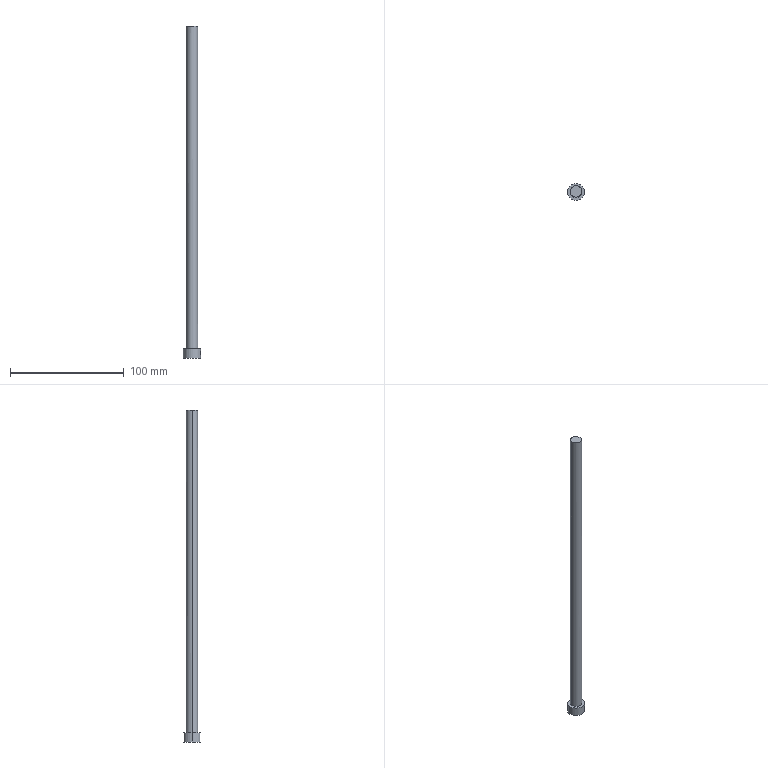Part | Creo | 1 solid | 10 faces | box 15 x 15 x 292.348 mm | volume 23678 mm3 | cylinder 6 | plane 4 | commonest cylinder face diameters 3 x2 10 x2 15 x2
STEP:
#1=CARTESIAN_POINT('',(85.,203.,-252.5));
#2=VERTEX_POINT('',#1);
#3=CARTESIAN_POINT('',(95.,203.,-252.5));
#4=VERTEX_POINT('',#3);
#5=CARTESIAN_POINT('',(90.,203.,-252.5));
#6=DIRECTION('',(0.,0.,-1.));
#7=DIRECTION('',(-1.,0.,0.));
#8=AXIS2_PLACEMENT_3D('',#5,#6,#7);
#9=CIRCLE('',#8,5.);
#10=EDGE_CURVE('',#2,#4,#9,.T.);
#11=ORIENTED_EDGE('',*,*,#10,.T.);
#12=CARTESIAN_POINT('',(95.,203.,31.466));
#13=VERTEX_POINT('',#12);
#14=CARTESIAN_POINT('',(95.,203.,31.466));
#15=DIRECTION('',(0.,0.,-1.));
#16=VECTOR('',#15,283.966);
#17=LINE('',#14,#16);
#18=EDGE_CURVE('',#13,#4,#17,.T.);
#19=ORIENTED_EDGE('',*,*,#18,.F.);
#20=CARTESIAN_POINT('',(85.,203.,31.848));
#21=VERTEX_POINT('',#20);
#22=CARTESIAN_POINT('',(95.,203.,31.466));
#23=CARTESIAN_POINT('',(95.,203.589,31.466));
#24=CARTESIAN_POINT('',(94.785,204.862,31.474));
#25=CARTESIAN_POINT('',(93.645,206.641,31.518));
#26=CARTESIAN_POINT('',(91.85,207.786,31.586));
#27=CARTESIAN_POINT('',(90.,208.107,31.657));
#28=CARTESIAN_POINT('',(88.15,207.786,31.727));
#29=CARTESIAN_POINT('',(86.355,206.641,31.796));
#30=CARTESIAN_POINT('',(85.215,204.862,31.839));
#31=CARTESIAN_POINT('',(85.,203.589,31.848));
#32=CARTESIAN_POINT('',(85.,203.,31.848));
#33=B_SPLINE_CURVE_WITH_KNOTS('',3,(#22,#23,#24,#25,#26,#27,#28,#29,#30,#31,#32),.UNSPECIFIED.,.F.,.F.,(4,1,1,1,1,1,1,1,4),(0.,0.125,0.25,0.375,0.5,0.625,0.75,0.875,1.),.UNSPECIFIED.);
#34=EDGE_CURVE('',#13,#21,#33,.T.);
#35=ORIENTED_EDGE('',*,*,#34,.T.);
#36=CARTESIAN_POINT('',(85.,203.,31.848));
#37=DIRECTION('',(0.,0.,-1.));
#38=VECTOR('',#37,284.348);
#39=LINE('',#36,#38);
#40=EDGE_CURVE('',#21,#2,#39,.T.);
#41=ORIENTED_EDGE('',*,*,#40,.T.);
#42=EDGE_LOOP('',(#11,#19,#35,#41));
#43=FACE_OUTER_BOUND('',#42,.F.);
#44=CARTESIAN_POINT('',(90.,203.,135.));
#45=DIRECTION('',(0.,0.,-1.));
#46=DIRECTION('',(-1.,0.,0.));
#47=AXIS2_PLACEMENT_3D('',#44,#45,#46);
#48=CYLINDRICAL_SURFACE('',#47,5.);
#49=ADVANCED_FACE('',(#43),#48,.T.);
#50=CARTESIAN_POINT('',(82.5,203.,-252.5));
#51=VERTEX_POINT('',#50);
#52=CARTESIAN_POINT('',(97.5,203.,-252.5));
#53=VERTEX_POINT('',#52);
#54=CARTESIAN_POINT('',(90.,203.,-252.5));
#55=DIRECTION('',(0.,0.,1.));
#56=DIRECTION('',(-1.,0.,0.));
#57=AXIS2_PLACEMENT_3D('',#54,#55,#56);
#58=CIRCLE('',#57,7.5);
#59=EDGE_CURVE('',#51,#53,#58,.T.);
#60=ORIENTED_EDGE('',*,*,#59,.F.);
#61=CARTESIAN_POINT('',(90.,203.,-252.5));
#62=DIRECTION('',(0.,0.,1.));
#63=DIRECTION('',(1.,0.,0.));
#64=AXIS2_PLACEMENT_3D('',#61,#62,#63);
#65=CIRCLE('',#64,7.5);
#66=EDGE_CURVE('',#53,#51,#65,.T.);
#67=ORIENTED_EDGE('',*,*,#66,.F.);
#68=EDGE_LOOP('',(#60,#67));
#69=FACE_OUTER_BOUND('',#68,.F.);
#70=ORIENTED_EDGE('',*,*,#10,.F.);
#71=CARTESIAN_POINT('',(90.,203.,-252.5));
#72=DIRECTION('',(0.,0.,-1.));
#73=DIRECTION('',(1.,0.,0.));
#74=AXIS2_PLACEMENT_3D('',#71,#72,#73);
#75=CIRCLE('',#74,5.);
#76=EDGE_CURVE('',#4,#2,#75,.T.);
#77=ORIENTED_EDGE('',*,*,#76,.F.);
#78=EDGE_LOOP('',(#70,#77));
#79=FACE_BOUND('',#78,.F.);
#80=CARTESIAN_POINT('',(90.,203.,-252.5));
#81=DIRECTION('',(0.,0.,1.));
#82=DIRECTION('',(-1.,0.,0.));
#83=AXIS2_PLACEMENT_3D('',#80,#81,#82);
#84=PLANE('',#83);
#85=ADVANCED_FACE('',(#69,#79),#84,.T.);
#86=ORIENTED_EDGE('',*,*,#76,.T.);
#87=ORIENTED_EDGE('',*,*,#40,.F.);
#88=CARTESIAN_POINT('',(85.,203.,31.848));
#89=CARTESIAN_POINT('',(85.,202.411,31.848));
#90=CARTESIAN_POINT('',(85.215,201.138,31.839));
#91=CARTESIAN_POINT('',(86.355,199.359,31.796));
#92=CARTESIAN_POINT('',(88.15,198.214,31.727));
#93=CARTESIAN_POINT('',(90.,197.893,31.657));
#94=CARTESIAN_POINT('',(91.85,198.214,31.586));
#95=CARTESIAN_POINT('',(93.645,199.359,31.518));
#96=CARTESIAN_POINT('',(94.785,201.138,31.474));
#97=CARTESIAN_POINT('',(95.,202.411,31.466));
#98=CARTESIAN_POINT('',(95.,203.,31.466));
#99=B_SPLINE_CURVE_WITH_KNOTS('',3,(#88,#89,#90,#91,#92,#93,#94,#95,#96,#97,#98),.UNSPECIFIED.,.F.,.F.,(4,1,1,1,1,1,1,1,4),(0.,0.125,0.25,0.375,0.5,0.625,0.75,0.875,1.),.UNSPECIFIED.);
#100=EDGE_CURVE('',#21,#13,#99,.T.);
#101=ORIENTED_EDGE('',*,*,#100,.T.);
#102=ORIENTED_EDGE('',*,*,#18,.T.);
#103=EDGE_LOOP('',(#86,#87,#101,#102));
#104=FACE_OUTER_BOUND('',#103,.F.);
#105=CARTESIAN_POINT('',(90.,203.,135.));
#106=DIRECTION('',(0.,0.,-1.));
#107=DIRECTION('',(-1.,0.,0.));
#108=AXIS2_PLACEMENT_3D('',#105,#106,#107);
#109=CYLINDRICAL_SURFACE('',#108,5.);
#110=ADVANCED_FACE('',(#104),#109,.T.);
#111=ORIENTED_EDGE('',*,*,#34,.F.);
#112=ORIENTED_EDGE('',*,*,#100,.F.);
#113=EDGE_LOOP('',(#111,#112));
#114=FACE_OUTER_BOUND('',#113,.F.);
#115=CARTESIAN_POINT('',(-122.791,-167.242,39.779));
#116=DIRECTION('',(-0.03814,0.,-0.9993));
#117=DIRECTION('',(-0.9993,0.,0.03814));
#118=AXIS2_PLACEMENT_3D('',#115,#116,#117);
#119=PLANE('',#118);
#120=ADVANCED_FACE('',(#114),#119,.F.);
#121=CARTESIAN_POINT('',(97.5,203.,-258.));
#122=VERTEX_POINT('',#121);
#123=CARTESIAN_POINT('',(97.5,203.,-255.));
#124=VERTEX_POINT('',#123);
#125=CARTESIAN_POINT('',(97.5,203.,-258.));
#126=CARTESIAN_POINT('',(97.5,202.795,-258.));
#127=CARTESIAN_POINT('',(97.484,202.417,-257.922));
#128=CARTESIAN_POINT('',(97.425,201.91,-257.589));
#129=CARTESIAN_POINT('',(97.365,201.576,-257.085));
#130=CARTESIAN_POINT('',(97.34,201.461,-256.497));
#131=CARTESIAN_POINT('',(97.365,201.578,-255.912));
#132=CARTESIAN_POINT('',(97.425,201.909,-255.413));
#133=CARTESIAN_POINT('',(97.484,202.415,-255.078));
#134=CARTESIAN_POINT('',(97.5,202.794,-255.));
#135=CARTESIAN_POINT('',(97.5,203.,-255.));
#136=B_SPLINE_CURVE_WITH_KNOTS('',3,(#125,#126,#127,#128,#129,#130,#131,#132,#133,#134,#135),.UNSPECIFIED.,.F.,.F.,(4,1,1,1,1,1,1,1,4),(0.,0.125,0.25,0.375,0.5,0.625,0.75,0.875,1.),.UNSPECIFIED.);
#137=EDGE_CURVE('',#122,#124,#136,.T.);
#138=ORIENTED_EDGE('',*,*,#137,.F.);
#139=CARTESIAN_POINT('',(97.5,203.,-260.5));
#140=VERTEX_POINT('',#139);
#141=CARTESIAN_POINT('',(97.5,203.,-260.5));
#142=DIRECTION('',(0.,0.,1.));
#143=VECTOR('',#142,2.5);
#144=LINE('',#141,#143);
#145=EDGE_CURVE('',#140,#122,#144,.T.);
#146=ORIENTED_EDGE('',*,*,#145,.F.);
#147=CARTESIAN_POINT('',(82.5,203.,-260.5));
#148=VERTEX_POINT('',#147);
#149=CARTESIAN_POINT('',(90.,203.,-260.5));
#150=DIRECTION('',(0.,0.,-1.));
#151=DIRECTION('',(1.,0.,0.));
#152=AXIS2_PLACEMENT_3D('',#149,#150,#151);
#153=CIRCLE('',#152,7.5);
#154=EDGE_CURVE('',#140,#148,#153,.T.);
#155=ORIENTED_EDGE('',*,*,#154,.T.);
#156=CARTESIAN_POINT('',(82.5,203.,-260.5));
#157=DIRECTION('',(0.,0.,1.));
#158=VECTOR('',#157,8.);
#159=LINE('',#156,#158);
#160=EDGE_CURVE('',#148,#51,#159,.T.);
#161=ORIENTED_EDGE('',*,*,#160,.T.);
#162=ORIENTED_EDGE('',*,*,#59,.T.);
#163=CARTESIAN_POINT('',(97.5,203.,-255.));
#164=DIRECTION('',(0.000005138,0.,1.));
#165=VECTOR('',#164,2.5);
#166=LINE('',#163,#165);
#167=EDGE_CURVE('',#124,#53,#166,.T.);
#168=ORIENTED_EDGE('',*,*,#167,.F.);
#169=EDGE_LOOP('',(#138,#146,#155,#161,#162,#168));
#170=FACE_OUTER_BOUND('',#169,.F.);
#171=CARTESIAN_POINT('',(90.,203.,-260.5));
#172=DIRECTION('',(0.,0.,1.));
#173=DIRECTION('',(-1.,0.,0.));
#174=AXIS2_PLACEMENT_3D('',#171,#172,#173);
#175=CYLINDRICAL_SURFACE('',#174,7.5);
#176=ADVANCED_FACE('',(#170),#175,.T.);
#177=ORIENTED_EDGE('',*,*,#137,.T.);
#178=CARTESIAN_POINT('',(90.,203.,-255.));
#179=VERTEX_POINT('',#178);
#180=CARTESIAN_POINT('',(90.,203.,-255.));
#181=DIRECTION('',(1.,0.,-0.000004561));
#182=VECTOR('',#181,7.5);
#183=LINE('',#180,#182);
#184=EDGE_CURVE('',#179,#124,#183,.T.);
#185=ORIENTED_EDGE('',*,*,#184,.F.);
#186=CARTESIAN_POINT('',(90.,203.,-258.));
#187=VERTEX_POINT('',#186);
#188=CARTESIAN_POINT('',(90.,203.,-256.5));
#189=DIRECTION('',(1.,0.,0.));
#190=DIRECTION('',(0.,0.,1.));
#191=AXIS2_PLACEMENT_3D('',#188,#189,#190);
#192=CIRCLE('',#191,1.5);
#193=EDGE_CURVE('',#179,#187,#192,.T.);
#194=ORIENTED_EDGE('',*,*,#193,.T.);
#195=CARTESIAN_POINT('',(90.,203.,-258.));
#196=DIRECTION('',(1.,0.,0.));
#197=VECTOR('',#196,7.5);
#198=LINE('',#195,#197);
#199=EDGE_CURVE('',#187,#122,#198,.T.);
#200=ORIENTED_EDGE('',*,*,#199,.T.);
#201=EDGE_LOOP('',(#177,#185,#194,#200));
#202=FACE_OUTER_BOUND('',#201,.F.);
#203=CARTESIAN_POINT('',(90.,203.,-256.5));
#204=DIRECTION('',(1.,0.,0.));
#205=DIRECTION('',(0.,0.,-1.));
#206=AXIS2_PLACEMENT_3D('',#203,#204,#205);
#207=CYLINDRICAL_SURFACE('',#206,1.5);
#208=ADVANCED_FACE('',(#202),#207,.F.);
#209=CARTESIAN_POINT('',(97.5,203.,-255.));
#210=CARTESIAN_POINT('',(97.5,203.206,-255.));
#211=CARTESIAN_POINT('',(97.484,203.585,-255.078));
#212=CARTESIAN_POINT('',(97.424,204.093,-255.414));
#213=CARTESIAN_POINT('',(97.364,204.424,-255.917));
#214=CARTESIAN_POINT('',(97.34,204.539,-256.506));
#215=CARTESIAN_POINT('',(97.365,204.421,-257.089));
#216=CARTESIAN_POINT('',(97.424,204.092,-257.586));
#217=CARTESIAN_POINT('',(97.484,203.586,-257.922));
#218=CARTESIAN_POINT('',(97.5,203.206,-258.));
#219=CARTESIAN_POINT('',(97.5,203.,-258.));
#220=B_SPLINE_CURVE_WITH_KNOTS('',3,(#209,#210,#211,#212,#213,#214,#215,#216,#217,#218,#219),.UNSPECIFIED.,.F.,.F.,(4,1,1,1,1,1,1,1,4),(0.,0.125,0.25,0.375,0.5,0.625,0.75,0.875,1.),.UNSPECIFIED.);
#221=EDGE_CURVE('',#124,#122,#220,.T.);
#222=ORIENTED_EDGE('',*,*,#221,.T.);
#223=ORIENTED_EDGE('',*,*,#199,.F.);
#224=CARTESIAN_POINT('',(90.,203.,-256.5));
#225=DIRECTION('',(1.,0.,0.));
#226=DIRECTION('',(0.,0.,-1.));
#227=AXIS2_PLACEMENT_3D('',#224,#225,#226);
#228=CIRCLE('',#227,1.5);
#229=EDGE_CURVE('',#187,#179,#228,.T.);
#230=ORIENTED_EDGE('',*,*,#229,.T.);
#231=ORIENTED_EDGE('',*,*,#184,.T.);
#232=EDGE_LOOP('',(#222,#223,#230,#231));
#233=FACE_OUTER_BOUND('',#232,.F.);
#234=CARTESIAN_POINT('',(90.,203.,-256.5));
#235=DIRECTION('',(1.,0.,0.));
#236=DIRECTION('',(0.,0.,-1.));
#237=AXIS2_PLACEMENT_3D('',#234,#235,#236);
#238=CYLINDRICAL_SURFACE('',#237,1.5);
#239=ADVANCED_FACE('',(#233),#238,.F.);
#240=ORIENTED_EDGE('',*,*,#221,.F.);
#241=ORIENTED_EDGE('',*,*,#167,.T.);
#242=ORIENTED_EDGE('',*,*,#66,.T.);
#243=ORIENTED_EDGE('',*,*,#160,.F.);
#244=CARTESIAN_POINT('',(90.,203.,-260.5));
#245=DIRECTION('',(0.,0.,-1.));
#246=DIRECTION('',(-1.,0.,0.));
#247=AXIS2_PLACEMENT_3D('',#244,#245,#246);
#248=CIRCLE('',#247,7.5);
#249=EDGE_CURVE('',#148,#140,#248,.T.);
#250=ORIENTED_EDGE('',*,*,#249,.T.);
#251=ORIENTED_EDGE('',*,*,#145,.T.);
#252=EDGE_LOOP('',(#240,#241,#242,#243,#250,#251));
#253=FACE_OUTER_BOUND('',#252,.F.);
#254=CARTESIAN_POINT('',(90.,203.,-260.5));
#255=DIRECTION('',(0.,0.,1.));
#256=DIRECTION('',(-1.,0.,0.));
#257=AXIS2_PLACEMENT_3D('',#254,#255,#256);
#258=CYLINDRICAL_SURFACE('',#257,7.5);
#259=ADVANCED_FACE('',(#253),#258,.T.);
#260=ORIENTED_EDGE('',*,*,#154,.F.);
#261=ORIENTED_EDGE('',*,*,#249,.F.);
#262=EDGE_LOOP('',(#260,#261));
#263=FACE_OUTER_BOUND('',#262,.F.);
#264=CARTESIAN_POINT('',(127.286,345.015,-260.5));
#265=DIRECTION('',(0.,0.,-1.));
#266=DIRECTION('',(1.,0.,0.));
#267=AXIS2_PLACEMENT_3D('',#264,#265,#266);
#268=PLANE('',#267);
#269=ADVANCED_FACE('',(#263),#268,.T.);
#270=ORIENTED_EDGE('',*,*,#229,.F.);
#271=ORIENTED_EDGE('',*,*,#193,.F.);
#272=EDGE_LOOP('',(#270,#271));
#273=FACE_OUTER_BOUND('',#272,.F.);
#274=CARTESIAN_POINT('',(90.,203.,-256.5));
#275=DIRECTION('',(-1.,0.,0.));
#276=DIRECTION('',(0.,0.,1.));
#277=AXIS2_PLACEMENT_3D('',#274,#275,#276);
#278=PLANE('',#277);
#279=ADVANCED_FACE('',(#273),#278,.F.);
#280=CLOSED_SHELL('',(#49,#85,#110,#120,#176,#208,#239,#259,#269,#279));
#281=MANIFOLD_SOLID_BREP('',#280);
#282=(LENGTH_UNIT()NAMED_UNIT(*)SI_UNIT(.MILLI.,.METRE.));
#283=UNCERTAINTY_MEASURE_WITH_UNIT(LENGTH_MEASURE(0.02931),#282,'','');
#284=(NAMED_UNIT(*)PLANE_ANGLE_UNIT()SI_UNIT($,.RADIAN.));
#285=PLANE_ANGLE_MEASURE_WITH_UNIT(PLANE_ANGLE_MEASURE(0.01745),#284);
#286=(CONVERSION_BASED_UNIT('DEGREE',#285)NAMED_UNIT(*)PLANE_ANGLE_UNIT());
#287=(NAMED_UNIT(*)SI_UNIT($,.STERADIAN.)SOLID_ANGLE_UNIT());
#288=(GEOMETRIC_REPRESENTATION_CONTEXT(3)GLOBAL_UNCERTAINTY_ASSIGNED_CONTEXT((#283))GLOBAL_UNIT_ASSIGNED_CONTEXT((#282,#286,#287))REPRESENTATION_CONTEXT('',''));
#289=ADVANCED_BREP_SHAPE_REPRESENTATION('',(#281),#288);